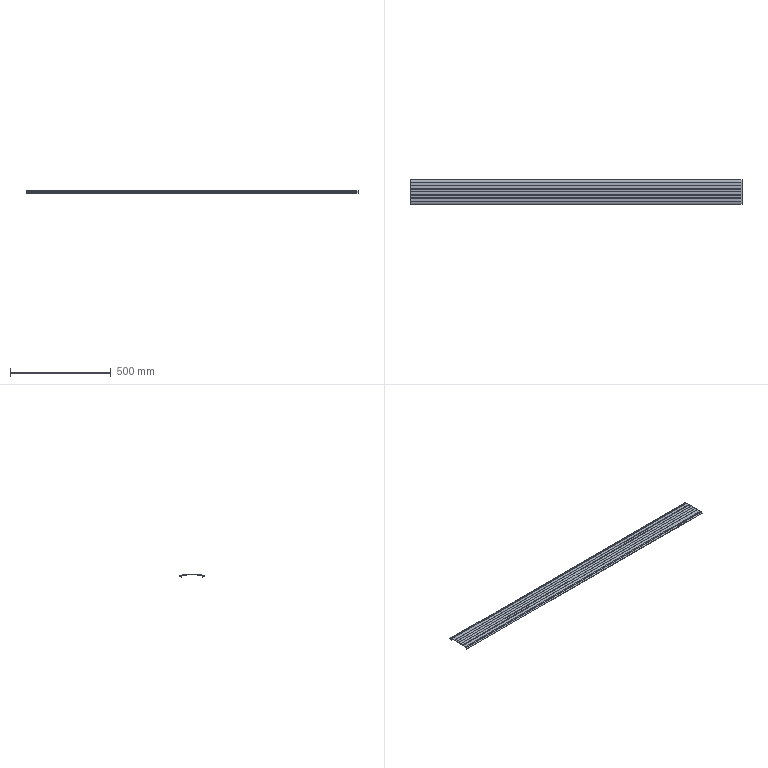Part | STEP file | 1 solid | 58 faces | box 1650 x 122.645 x 13.207 mm | volume 270111 mm3 | cylinder 30 | plane 28 | commonest cylinder face diameters 0.4 x7 2001 x6 2 x4 58.3 x4 20 x2 60.6 x2